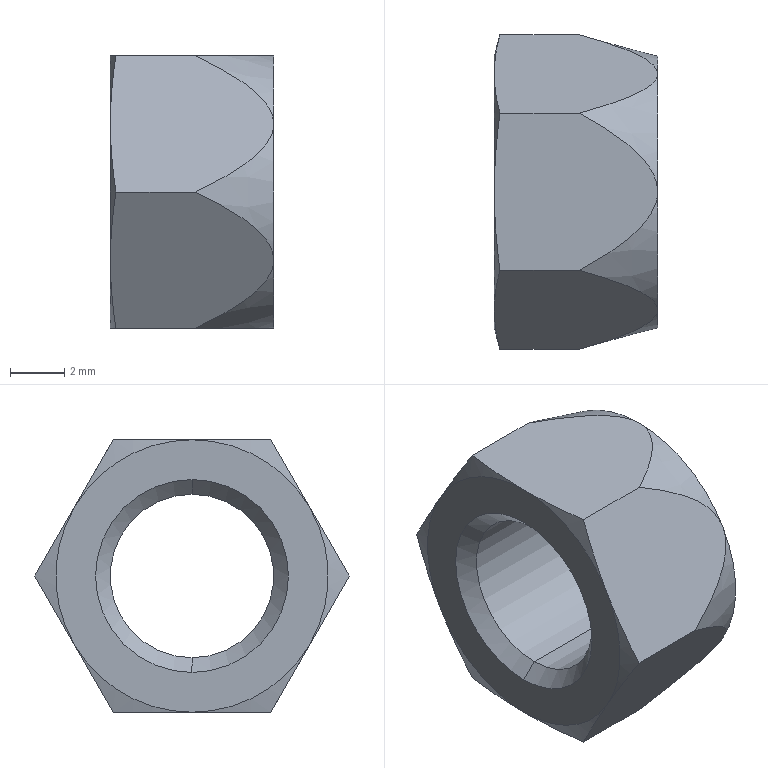Part | STEP file | Microwave Drying Flat Conveyor-nut_gb_t_6185_1_m6 | 1 solid | 26 faces | box 6 x 11.547 x 10 mm | volume 336.581 mm3 | cone 16 | plane 8 | cylinder 2 | commonest cylinder face diameters 6 x2
STEP:
#1=CARTESIAN_POINT('',(0.5413,0.,-3.));
#2=VERTEX_POINT('',#1);
#3=CARTESIAN_POINT('',(0.5413,0.,3.));
#4=VERTEX_POINT('',#3);
#5=CARTESIAN_POINT('',(0.5413,0.,0.));
#6=DIRECTION('',(-1.,0.,0.));
#7=DIRECTION('',(0.,0.,1.));
#8=AXIS2_PLACEMENT_3D('',#5,#6,#7);
#9=CIRCLE('',#8,3.);
#10=EDGE_CURVE('',#2,#4,#9,.T.);
#11=ORIENTED_EDGE('',*,*,#10,.F.);
#12=CARTESIAN_POINT('',(0.,0.,-3.541));
#13=VERTEX_POINT('',#12);
#14=CARTESIAN_POINT('',(0.,0.,-3.541));
#15=DIRECTION('',(-0.7071,0.,-0.7071));
#16=VECTOR('',#15,1000.);
#17=LINE('',#14,#16);
#18=EDGE_CURVE('',#2,#13,#17,.T.);
#19=ORIENTED_EDGE('',*,*,#18,.T.);
#20=CARTESIAN_POINT('',(0.,0.,3.541));
#21=VERTEX_POINT('',#20);
#22=CARTESIAN_POINT('',(0.,0.,0.));
#23=DIRECTION('',(-1.,0.,0.));
#24=DIRECTION('',(0.,0.,1.));
#25=AXIS2_PLACEMENT_3D('',#22,#23,#24);
#26=CIRCLE('',#25,3.541);
#27=EDGE_CURVE('',#13,#21,#26,.T.);
#28=ORIENTED_EDGE('',*,*,#27,.T.);
#29=CARTESIAN_POINT('',(0.,0.,3.541));
#30=DIRECTION('',(-0.7071,0.,0.7071));
#31=VECTOR('',#30,1000.);
#32=LINE('',#29,#31);
#33=EDGE_CURVE('',#4,#21,#32,.T.);
#34=ORIENTED_EDGE('',*,*,#33,.F.);
#35=EDGE_LOOP('',(#11,#19,#28,#34));
#36=FACE_OUTER_BOUND('',#35,.T.);
#37=CARTESIAN_POINT('',(0.,0.,0.));
#38=DIRECTION('',(-1.,0.,0.));
#39=DIRECTION('',(0.,0.,1.));
#40=AXIS2_PLACEMENT_3D('',#37,#38,#39);
#41=CONICAL_SURFACE('',#40,3.541,0.7854);
#42=ADVANCED_FACE('',(#36),#41,.F.);
#43=CARTESIAN_POINT('',(5.459,0.,-3.));
#44=VERTEX_POINT('',#43);
#45=CARTESIAN_POINT('',(5.459,0.,3.));
#46=VERTEX_POINT('',#45);
#47=CARTESIAN_POINT('',(5.459,0.,0.));
#48=DIRECTION('',(-1.,0.,0.));
#49=DIRECTION('',(0.,0.,1.));
#50=AXIS2_PLACEMENT_3D('',#47,#48,#49);
#51=CIRCLE('',#50,3.);
#52=EDGE_CURVE('',#44,#46,#51,.T.);
#53=ORIENTED_EDGE('',*,*,#52,.F.);
#54=CARTESIAN_POINT('',(0.,0.,-3.));
#55=DIRECTION('',(-1.,0.,0.));
#56=VECTOR('',#55,1000.);
#57=LINE('',#54,#56);
#58=EDGE_CURVE('',#44,#2,#57,.T.);
#59=ORIENTED_EDGE('',*,*,#58,.T.);
#60=ORIENTED_EDGE('',*,*,#10,.T.);
#61=CARTESIAN_POINT('',(0.,0.,3.));
#62=DIRECTION('',(-1.,0.,0.));
#63=VECTOR('',#62,1000.);
#64=LINE('',#61,#63);
#65=EDGE_CURVE('',#46,#4,#64,.T.);
#66=ORIENTED_EDGE('',*,*,#65,.F.);
#67=EDGE_LOOP('',(#53,#59,#60,#66));
#68=FACE_OUTER_BOUND('',#67,.T.);
#69=CARTESIAN_POINT('',(0.,0.,0.));
#70=DIRECTION('',(-1.,0.,0.));
#71=DIRECTION('',(0.,0.,1.));
#72=AXIS2_PLACEMENT_3D('',#69,#70,#71);
#73=CYLINDRICAL_SURFACE('',#72,3.);
#74=ADVANCED_FACE('',(#68),#73,.F.);
#75=ORIENTED_EDGE('',*,*,#52,.T.);
#76=CARTESIAN_POINT('',(6.,0.,3.541));
#77=VERTEX_POINT('',#76);
#78=CARTESIAN_POINT('',(5.459,0.,3.));
#79=DIRECTION('',(0.7071,0.,0.7071));
#80=VECTOR('',#79,1000.);
#81=LINE('',#78,#80);
#82=EDGE_CURVE('',#46,#77,#81,.T.);
#83=ORIENTED_EDGE('',*,*,#82,.T.);
#84=CARTESIAN_POINT('',(6.,0.,-3.541));
#85=VERTEX_POINT('',#84);
#86=CARTESIAN_POINT('',(6.,0.,0.));
#87=DIRECTION('',(-1.,0.,0.));
#88=DIRECTION('',(0.,0.,1.));
#89=AXIS2_PLACEMENT_3D('',#86,#87,#88);
#90=CIRCLE('',#89,3.541);
#91=EDGE_CURVE('',#85,#77,#90,.T.);
#92=ORIENTED_EDGE('',*,*,#91,.F.);
#93=CARTESIAN_POINT('',(5.459,0.,-3.));
#94=DIRECTION('',(0.7071,0.,-0.7071));
#95=VECTOR('',#94,1000.);
#96=LINE('',#93,#95);
#97=EDGE_CURVE('',#44,#85,#96,.T.);
#98=ORIENTED_EDGE('',*,*,#97,.F.);
#99=EDGE_LOOP('',(#75,#83,#92,#98));
#100=FACE_OUTER_BOUND('',#99,.T.);
#101=CARTESIAN_POINT('',(5.459,0.,0.));
#102=DIRECTION('',(1.,0.,0.));
#103=DIRECTION('',(0.,0.,-1.));
#104=AXIS2_PLACEMENT_3D('',#101,#102,#103);
#105=CONICAL_SURFACE('',#104,3.,0.7854);
#106=ADVANCED_FACE('',(#100),#105,.F.);
#107=CARTESIAN_POINT('',(3.113,2.887,-5.));
#108=VERTEX_POINT('',#107);
#109=CARTESIAN_POINT('',(6.,0.,-5.));
#110=VERTEX_POINT('',#109);
#111=CARTESIAN_POINT('',(3.113,2.887,-5.));
#112=CARTESIAN_POINT('',(3.423,2.721,-5.));
#113=CARTESIAN_POINT('',(3.729,2.547,-5.));
#114=CARTESIAN_POINT('',(4.326,2.172,-5.));
#115=CARTESIAN_POINT('',(4.619,1.97,-5.));
#116=CARTESIAN_POINT('',(5.033,1.634,-5.));
#117=CARTESIAN_POINT('',(5.165,1.517,-5.));
#118=CARTESIAN_POINT('',(5.416,1.267,-5.));
#119=CARTESIAN_POINT('',(5.534,1.133,-5.));
#120=CARTESIAN_POINT('',(5.744,0.8433,-5.));
#121=CARTESIAN_POINT('',(5.833,0.69,-5.));
#122=CARTESIAN_POINT('',(5.963,0.3563,-5.));
#123=CARTESIAN_POINT('',(6.,0.1802,-5.));
#124=CARTESIAN_POINT('',(6.,0.,-5.));
#125=B_SPLINE_CURVE_WITH_KNOTS('',3,(#111,#112,#113,#114,#115,#116,#117,#118,#119,#120,#121,#122,#123,#124),.UNSPECIFIED.,.F.,.F.,(4,2,2,2,2,2,4),(0.002995,0.004049,0.005104,0.005631,0.006158,0.006685,0.007212),.UNSPECIFIED.);
#126=EDGE_CURVE('',#108,#110,#125,.T.);
#127=ORIENTED_EDGE('',*,*,#126,.F.);
#128=CARTESIAN_POINT('',(6.,4.33,-2.5));
#129=VERTEX_POINT('',#128);
#130=CARTESIAN_POINT('',(6.,4.33,-2.5));
#131=CARTESIAN_POINT('',(6.,4.241,-2.654));
#132=CARTESIAN_POINT('',(5.963,4.152,-2.808));
#133=CARTESIAN_POINT('',(5.835,3.987,-3.095));
#134=CARTESIAN_POINT('',(5.745,3.909,-3.229));
#135=CARTESIAN_POINT('',(5.432,3.693,-3.604));
#136=CARTESIAN_POINT('',(5.174,3.571,-3.816));
#137=CARTESIAN_POINT('',(4.623,3.346,-4.204));
#138=CARTESIAN_POINT('',(4.331,3.246,-4.378));
#139=CARTESIAN_POINT('',(3.733,3.058,-4.703));
#140=CARTESIAN_POINT('',(3.426,2.97,-4.855));
#141=CARTESIAN_POINT('',(3.113,2.887,-5.));
#142=B_SPLINE_CURVE_WITH_KNOTS('',3,(#130,#131,#132,#133,#134,#135,#136,#137,#138,#139,#140,#141),.UNSPECIFIED.,.F.,.F.,(4,2,2,2,2,4),(0.004244,0.004777,0.005309,0.006373,0.007438,0.008503),.UNSPECIFIED.);
#143=EDGE_CURVE('',#129,#108,#142,.T.);
#144=ORIENTED_EDGE('',*,*,#143,.F.);
#145=CARTESIAN_POINT('',(6.,0.,0.));
#146=DIRECTION('',(-1.,0.,0.));
#147=DIRECTION('',(0.,0.,1.));
#148=AXIS2_PLACEMENT_3D('',#145,#146,#147);
#149=CIRCLE('',#148,5.);
#150=EDGE_CURVE('',#129,#110,#149,.T.);
#151=ORIENTED_EDGE('',*,*,#150,.T.);
#152=EDGE_LOOP('',(#127,#144,#151));
#153=FACE_OUTER_BOUND('',#152,.T.);
#154=CARTESIAN_POINT('',(6.,0.,0.));
#155=DIRECTION('',(-1.,0.,0.));
#156=DIRECTION('',(0.,0.,1.));
#157=AXIS2_PLACEMENT_3D('',#154,#155,#156);
#158=CONICAL_SURFACE('',#157,5.,0.2618);
#159=ADVANCED_FACE('',(#153),#158,.T.);
#160=CARTESIAN_POINT('',(3.113,-2.887,-5.));
#161=VERTEX_POINT('',#160);
#162=CARTESIAN_POINT('',(6.,0.,-5.));
#163=CARTESIAN_POINT('',(6.,-0.1814,-5.));
#164=CARTESIAN_POINT('',(5.962,-0.3586,-5.));
#165=CARTESIAN_POINT('',(5.831,-0.6949,-5.));
#166=CARTESIAN_POINT('',(5.74,-0.8495,-5.));
#167=CARTESIAN_POINT('',(5.527,-1.142,-5.));
#168=CARTESIAN_POINT('',(5.409,-1.274,-5.));
#169=CARTESIAN_POINT('',(5.16,-1.522,-5.));
#170=CARTESIAN_POINT('',(5.028,-1.638,-5.));
#171=CARTESIAN_POINT('',(4.62,-1.969,-5.));
#172=CARTESIAN_POINT('',(4.33,-2.169,-5.));
#173=CARTESIAN_POINT('',(3.731,-2.545,-5.));
#174=CARTESIAN_POINT('',(3.423,-2.721,-5.));
#175=CARTESIAN_POINT('',(3.113,-2.887,-5.));
#176=B_SPLINE_CURVE_WITH_KNOTS('',3,(#162,#163,#164,#165,#166,#167,#168,#169,#170,#171,#172,#173,#174,#175),.UNSPECIFIED.,.F.,.F.,(4,2,2,2,2,2,4),(0.007212,0.007743,0.008274,0.008805,0.009335,0.0104,0.01146),.UNSPECIFIED.);
#177=EDGE_CURVE('',#110,#161,#176,.T.);
#178=ORIENTED_EDGE('',*,*,#177,.F.);
#179=CARTESIAN_POINT('',(6.,-4.33,-2.5));
#180=VERTEX_POINT('',#179);
#181=CARTESIAN_POINT('',(6.,0.,0.));
#182=DIRECTION('',(-1.,0.,0.));
#183=DIRECTION('',(0.,0.,1.));
#184=AXIS2_PLACEMENT_3D('',#181,#182,#183);
#185=CIRCLE('',#184,5.);
#186=EDGE_CURVE('',#110,#180,#185,.T.);
#187=ORIENTED_EDGE('',*,*,#186,.T.);
#188=CARTESIAN_POINT('',(3.113,-2.887,-5.));
#189=CARTESIAN_POINT('',(3.426,-2.97,-4.855));
#190=CARTESIAN_POINT('',(3.733,-3.058,-4.703));
#191=CARTESIAN_POINT('',(4.332,-3.246,-4.377));
#192=CARTESIAN_POINT('',(4.625,-3.347,-4.203));
#193=CARTESIAN_POINT('',(5.037,-3.515,-3.912));
#194=CARTESIAN_POINT('',(5.17,-3.574,-3.81));
#195=CARTESIAN_POINT('',(5.42,-3.699,-3.593));
#196=CARTESIAN_POINT('',(5.539,-3.766,-3.476));
#197=CARTESIAN_POINT('',(5.745,-3.91,-3.228));
#198=CARTESIAN_POINT('',(5.835,-3.987,-3.094));
#199=CARTESIAN_POINT('',(5.931,-4.111,-2.879));
#200=CARTESIAN_POINT('',(5.956,-4.154,-2.805));
#201=CARTESIAN_POINT('',(5.991,-4.241,-2.655));
#202=CARTESIAN_POINT('',(6.,-4.286,-2.577));
#203=CARTESIAN_POINT('',(6.,-4.33,-2.5));
#204=B_SPLINE_CURVE_WITH_KNOTS('',3,(#188,#189,#190,#191,#192,#193,#194,#195,#196,#197,#198,#199,#200,#201,#202,#203),.UNSPECIFIED.,.F.,.F.,(4,2,2,2,2,2,2,4),(0.000000005,0.001061,0.002122,0.002653,0.003183,0.003714,0.003979,0.004244),.UNSPECIFIED.);
#205=EDGE_CURVE('',#161,#180,#204,.T.);
#206=ORIENTED_EDGE('',*,*,#205,.F.);
#207=EDGE_LOOP('',(#178,#187,#206));
#208=FACE_OUTER_BOUND('',#207,.T.);
#209=CARTESIAN_POINT('',(6.,0.,0.));
#210=DIRECTION('',(-1.,0.,0.));
#211=DIRECTION('',(0.,0.,1.));
#212=AXIS2_PLACEMENT_3D('',#209,#210,#211);
#213=CONICAL_SURFACE('',#212,5.,0.2618);
#214=ADVANCED_FACE('',(#208),#213,.T.);
#215=CARTESIAN_POINT('',(3.113,-5.774,0.));
#216=VERTEX_POINT('',#215);
#217=CARTESIAN_POINT('',(6.,-4.33,-2.5));
#218=CARTESIAN_POINT('',(6.,-4.419,-2.346));
#219=CARTESIAN_POINT('',(5.963,-4.508,-2.192));
#220=CARTESIAN_POINT('',(5.835,-4.674,-1.905));
#221=CARTESIAN_POINT('',(5.745,-4.751,-1.771));
#222=CARTESIAN_POINT('',(5.432,-4.968,-1.396));
#223=CARTESIAN_POINT('',(5.174,-5.09,-1.184));
#224=CARTESIAN_POINT('',(4.623,-5.314,-0.7959));
#225=CARTESIAN_POINT('',(4.331,-5.414,-0.6225));
#226=CARTESIAN_POINT('',(3.733,-5.602,-0.2968));
#227=CARTESIAN_POINT('',(3.426,-5.69,-0.145));
#228=CARTESIAN_POINT('',(3.113,-5.774,0.));
#229=B_SPLINE_CURVE_WITH_KNOTS('',3,(#217,#218,#219,#220,#221,#222,#223,#224,#225,#226,#227,#228),.UNSPECIFIED.,.F.,.F.,(4,2,2,2,2,4),(0.004244,0.004777,0.005309,0.006373,0.007438,0.008503),.UNSPECIFIED.);
#230=EDGE_CURVE('',#180,#216,#229,.T.);
#231=ORIENTED_EDGE('',*,*,#230,.F.);
#232=CARTESIAN_POINT('',(6.,-4.33,2.5));
#233=VERTEX_POINT('',#232);
#234=CARTESIAN_POINT('',(6.,0.,0.));
#235=DIRECTION('',(-1.,0.,0.));
#236=DIRECTION('',(0.,0.,1.));
#237=AXIS2_PLACEMENT_3D('',#234,#235,#236);
#238=CIRCLE('',#237,5.);
#239=EDGE_CURVE('',#180,#233,#238,.T.);
#240=ORIENTED_EDGE('',*,*,#239,.T.);
#241=CARTESIAN_POINT('',(3.113,-5.774,0.));
#242=CARTESIAN_POINT('',(3.426,-5.69,0.145));
#243=CARTESIAN_POINT('',(3.733,-5.602,0.2969));
#244=CARTESIAN_POINT('',(4.332,-5.414,0.623));
#245=CARTESIAN_POINT('',(4.625,-5.313,0.7973));
#246=CARTESIAN_POINT('',(5.037,-5.145,1.088));
#247=CARTESIAN_POINT('',(5.17,-5.086,1.19));
#248=CARTESIAN_POINT('',(5.42,-4.961,1.407));
#249=CARTESIAN_POINT('',(5.539,-4.894,1.524));
#250=CARTESIAN_POINT('',(5.745,-4.751,1.772));
#251=CARTESIAN_POINT('',(5.835,-4.673,1.906));
#252=CARTESIAN_POINT('',(5.931,-4.549,2.121));
#253=CARTESIAN_POINT('',(5.956,-4.506,2.195));
#254=CARTESIAN_POINT('',(5.991,-4.419,2.345));
#255=CARTESIAN_POINT('',(6.,-4.374,2.423));
#256=CARTESIAN_POINT('',(6.,-4.33,2.5));
#257=B_SPLINE_CURVE_WITH_KNOTS('',3,(#241,#242,#243,#244,#245,#246,#247,#248,#249,#250,#251,#252,#253,#254,#255,#256),.UNSPECIFIED.,.F.,.F.,(4,2,2,2,2,2,2,4),(0.000000005,0.001061,0.002122,0.002653,0.003183,0.003714,0.003979,0.004244),.UNSPECIFIED.);
#258=EDGE_CURVE('',#216,#233,#257,.T.);
#259=ORIENTED_EDGE('',*,*,#258,.F.);
#260=EDGE_LOOP('',(#231,#240,#259));
#261=FACE_OUTER_BOUND('',#260,.T.);
#262=CARTESIAN_POINT('',(6.,0.,0.));
#263=DIRECTION('',(-1.,0.,0.));
#264=DIRECTION('',(0.,0.,1.));
#265=AXIS2_PLACEMENT_3D('',#262,#263,#264);
#266=CONICAL_SURFACE('',#265,5.,0.2618);
#267=ADVANCED_FACE('',(#261),#266,.T.);
#268=CARTESIAN_POINT('',(3.113,5.774,0.));
#269=VERTEX_POINT('',#268);
#270=CARTESIAN_POINT('',(3.113,5.774,0.));
#271=CARTESIAN_POINT('',(3.426,5.69,-0.145));
#272=CARTESIAN_POINT('',(3.733,5.602,-0.2969));
#273=CARTESIAN_POINT('',(4.332,5.414,-0.623));
#274=CARTESIAN_POINT('',(4.625,5.313,-0.7973));
#275=CARTESIAN_POINT('',(5.037,5.145,-1.088));
#276=CARTESIAN_POINT('',(5.17,5.086,-1.19));
#277=CARTESIAN_POINT('',(5.42,4.961,-1.407));
#278=CARTESIAN_POINT('',(5.539,4.894,-1.524));
#279=CARTESIAN_POINT('',(5.745,4.751,-1.772));
#280=CARTESIAN_POINT('',(5.835,4.673,-1.906));
#281=CARTESIAN_POINT('',(5.931,4.549,-2.121));
#282=CARTESIAN_POINT('',(5.956,4.506,-2.195));
#283=CARTESIAN_POINT('',(5.991,4.419,-2.345));
#284=CARTESIAN_POINT('',(6.,4.374,-2.423));
#285=CARTESIAN_POINT('',(6.,4.33,-2.5));
#286=B_SPLINE_CURVE_WITH_KNOTS('',3,(#270,#271,#272,#273,#274,#275,#276,#277,#278,#279,#280,#281,#282,#283,#284,#285),.UNSPECIFIED.,.F.,.F.,(4,2,2,2,2,2,2,4),(0.000000005,0.001061,0.002122,0.002653,0.003183,0.003714,0.003979,0.004244),.UNSPECIFIED.);
#287=EDGE_CURVE('',#269,#129,#286,.T.);
#288=ORIENTED_EDGE('',*,*,#287,.F.);
#289=CARTESIAN_POINT('',(6.,4.33,2.5));
#290=VERTEX_POINT('',#289);
#291=CARTESIAN_POINT('',(6.,4.33,2.5));
#292=CARTESIAN_POINT('',(6.,4.419,2.346));
#293=CARTESIAN_POINT('',(5.963,4.508,2.192));
#294=CARTESIAN_POINT('',(5.835,4.674,1.905));
#295=CARTESIAN_POINT('',(5.745,4.751,1.771));
#296=CARTESIAN_POINT('',(5.432,4.968,1.396));
#297=CARTESIAN_POINT('',(5.174,5.09,1.184));
#298=CARTESIAN_POINT('',(4.623,5.314,0.7959));
#299=CARTESIAN_POINT('',(4.331,5.414,0.6225));
#300=CARTESIAN_POINT('',(3.733,5.602,0.2968));
#301=CARTESIAN_POINT('',(3.426,5.69,0.145));
#302=CARTESIAN_POINT('',(3.113,5.774,0.));
#303=B_SPLINE_CURVE_WITH_KNOTS('',3,(#291,#292,#293,#294,#295,#296,#297,#298,#299,#300,#301,#302),.UNSPECIFIED.,.F.,.F.,(4,2,2,2,2,4),(0.004244,0.004777,0.005309,0.006373,0.007438,0.008503),.UNSPECIFIED.);
#304=EDGE_CURVE('',#290,#269,#303,.T.);
#305=ORIENTED_EDGE('',*,*,#304,.F.);
#306=CARTESIAN_POINT('',(6.,0.,0.));
#307=DIRECTION('',(-1.,0.,0.));
#308=DIRECTION('',(0.,0.,1.));
#309=AXIS2_PLACEMENT_3D('',#306,#307,#308);
#310=CIRCLE('',#309,5.);
#311=EDGE_CURVE('',#290,#129,#310,.T.);
#312=ORIENTED_EDGE('',*,*,#311,.T.);
#313=EDGE_LOOP('',(#288,#305,#312));
#314=FACE_OUTER_BOUND('',#313,.T.);
#315=CARTESIAN_POINT('',(6.,0.,0.));
#316=DIRECTION('',(-1.,0.,0.));
#317=DIRECTION('',(0.,0.,1.));
#318=AXIS2_PLACEMENT_3D('',#315,#316,#317);
#319=CONICAL_SURFACE('',#318,5.,0.2618);
#320=ADVANCED_FACE('',(#314),#319,.T.);
#321=CARTESIAN_POINT('',(3.113,-2.887,5.));
#322=VERTEX_POINT('',#321);
#323=CARTESIAN_POINT('',(6.,-4.33,2.5));
#324=CARTESIAN_POINT('',(6.,-4.241,2.654));
#325=CARTESIAN_POINT('',(5.963,-4.152,2.808));
#326=CARTESIAN_POINT('',(5.835,-3.987,3.095));
#327=CARTESIAN_POINT('',(5.745,-3.909,3.229));
#328=CARTESIAN_POINT('',(5.432,-3.693,3.604));
#329=CARTESIAN_POINT('',(5.174,-3.571,3.816));
#330=CARTESIAN_POINT('',(4.623,-3.346,4.204));
#331=CARTESIAN_POINT('',(4.331,-3.246,4.378));
#332=CARTESIAN_POINT('',(3.733,-3.058,4.703));
#333=CARTESIAN_POINT('',(3.426,-2.97,4.855));
#334=CARTESIAN_POINT('',(3.113,-2.887,5.));
#335=B_SPLINE_CURVE_WITH_KNOTS('',3,(#323,#324,#325,#326,#327,#328,#329,#330,#331,#332,#333,#334),.UNSPECIFIED.,.F.,.F.,(4,2,2,2,2,4),(0.004244,0.004777,0.005309,0.006373,0.007438,0.008503),.UNSPECIFIED.);
#336=EDGE_CURVE('',#233,#322,#335,.T.);
#337=ORIENTED_EDGE('',*,*,#336,.F.);
#338=CARTESIAN_POINT('',(6.,0.,5.));
#339=VERTEX_POINT('',#338);
#340=CARTESIAN_POINT('',(6.,0.,0.));
#341=DIRECTION('',(-1.,0.,0.));
#342=DIRECTION('',(0.,0.,1.));
#343=AXIS2_PLACEMENT_3D('',#340,#341,#342);
#344=CIRCLE('',#343,5.);
#345=EDGE_CURVE('',#233,#339,#344,.T.);
#346=ORIENTED_EDGE('',*,*,#345,.T.);
#347=CARTESIAN_POINT('',(3.113,-2.887,5.));
#348=CARTESIAN_POINT('',(3.423,-2.721,5.));
#349=CARTESIAN_POINT('',(3.731,-2.545,5.));
#350=CARTESIAN_POINT('',(4.33,-2.169,5.));
#351=CARTESIAN_POINT('',(4.62,-1.969,5.));
#352=CARTESIAN_POINT('',(5.028,-1.638,5.));
#353=CARTESIAN_POINT('',(5.16,-1.522,5.));
#354=CARTESIAN_POINT('',(5.409,-1.274,5.));
#355=CARTESIAN_POINT('',(5.527,-1.142,5.));
#356=CARTESIAN_POINT('',(5.74,-0.8495,5.));
#357=CARTESIAN_POINT('',(5.831,-0.6949,5.));
#358=CARTESIAN_POINT('',(5.962,-0.3586,5.));
#359=CARTESIAN_POINT('',(6.,-0.1814,5.));
#360=CARTESIAN_POINT('',(6.,0.,5.));
#361=B_SPLINE_CURVE_WITH_KNOTS('',3,(#347,#348,#349,#350,#351,#352,#353,#354,#355,#356,#357,#358,#359,#360),.UNSPECIFIED.,.F.,.F.,(4,2,2,2,2,2,4),(0.008,0.009052,0.0101,0.01063,0.01115,0.01168,0.01221),.UNSPECIFIED.);
#362=EDGE_CURVE('',#322,#339,#361,.T.);
#363=ORIENTED_EDGE('',*,*,#362,.F.);
#364=EDGE_LOOP('',(#337,#346,#363));
#365=FACE_OUTER_BOUND('',#364,.T.);
#366=CARTESIAN_POINT('',(6.,0.,0.));
#367=DIRECTION('',(-1.,0.,0.));
#368=DIRECTION('',(0.,0.,1.));
#369=AXIS2_PLACEMENT_3D('',#366,#367,#368);
#370=CONICAL_SURFACE('',#369,5.,0.2618);
#371=ADVANCED_FACE('',(#365),#370,.T.);
#372=CARTESIAN_POINT('',(3.113,2.887,5.));
#373=VERTEX_POINT('',#372);
#374=CARTESIAN_POINT('',(3.113,2.887,5.));
#375=CARTESIAN_POINT('',(3.426,2.97,4.855));
#376=CARTESIAN_POINT('',(3.733,3.058,4.703));
#377=CARTESIAN_POINT('',(4.332,3.246,4.377));
#378=CARTESIAN_POINT('',(4.625,3.347,4.203));
#379=CARTESIAN_POINT('',(5.037,3.515,3.912));
#380=CARTESIAN_POINT('',(5.17,3.574,3.81));
#381=CARTESIAN_POINT('',(5.42,3.699,3.593));
#382=CARTESIAN_POINT('',(5.539,3.766,3.476));
#383=CARTESIAN_POINT('',(5.745,3.91,3.228));
#384=CARTESIAN_POINT('',(5.835,3.987,3.094));
#385=CARTESIAN_POINT('',(5.931,4.111,2.879));
#386=CARTESIAN_POINT('',(5.956,4.154,2.805));
#387=CARTESIAN_POINT('',(5.991,4.241,2.655));
#388=CARTESIAN_POINT('',(6.,4.286,2.577));
#389=CARTESIAN_POINT('',(6.,4.33,2.5));
#390=B_SPLINE_CURVE_WITH_KNOTS('',3,(#374,#375,#376,#377,#378,#379,#380,#381,#382,#383,#384,#385,#386,#387,#388,#389),.UNSPECIFIED.,.F.,.F.,(4,2,2,2,2,2,2,4),(0.000000005,0.001061,0.002122,0.002653,0.003183,0.003714,0.003979,0.004244),.UNSPECIFIED.);
#391=EDGE_CURVE('',#373,#290,#390,.T.);
#392=ORIENTED_EDGE('',*,*,#391,.F.);
#393=CARTESIAN_POINT('',(6.,0.,5.));
#394=CARTESIAN_POINT('',(6.,0.1802,5.));
#395=CARTESIAN_POINT('',(5.963,0.3563,5.));
#396=CARTESIAN_POINT('',(5.833,0.69,5.));
#397=CARTESIAN_POINT('',(5.744,0.8433,5.));
#398=CARTESIAN_POINT('',(5.534,1.133,5.));
#399=CARTESIAN_POINT('',(5.416,1.267,5.));
#400=CARTESIAN_POINT('',(5.165,1.517,5.));
#401=CARTESIAN_POINT('',(5.033,1.634,5.));
#402=CARTESIAN_POINT('',(4.619,1.97,5.));
#403=CARTESIAN_POINT('',(4.326,2.172,5.));
#404=CARTESIAN_POINT('',(3.729,2.547,5.));
#405=CARTESIAN_POINT('',(3.423,2.721,5.));
#406=CARTESIAN_POINT('',(3.113,2.887,5.));
#407=B_SPLINE_CURVE_WITH_KNOTS('',3,(#393,#394,#395,#396,#397,#398,#399,#400,#401,#402,#403,#404,#405,#406),.UNSPECIFIED.,.F.,.F.,(4,2,2,2,2,2,4),(0.01221,0.01273,0.01325,0.01377,0.01429,0.01534,0.01638),.UNSPECIFIED.);
#408=EDGE_CURVE('',#339,#373,#407,.T.);
#409=ORIENTED_EDGE('',*,*,#408,.F.);
#410=CARTESIAN_POINT('',(6.,0.,0.));
#411=DIRECTION('',(-1.,0.,0.));
#412=DIRECTION('',(0.,0.,1.));
#413=AXIS2_PLACEMENT_3D('',#410,#411,#412);
#414=CIRCLE('',#413,5.);
#415=EDGE_CURVE('',#339,#290,#414,.T.);
#416=ORIENTED_EDGE('',*,*,#415,.T.);
#417=EDGE_LOOP('',(#392,#409,#416));
#418=FACE_OUTER_BOUND('',#417,.T.);
#419=CARTESIAN_POINT('',(6.,0.,0.));
#420=DIRECTION('',(-1.,0.,0.));
#421=DIRECTION('',(0.,0.,1.));
#422=AXIS2_PLACEMENT_3D('',#419,#420,#421);
#423=CONICAL_SURFACE('',#422,5.,0.2618);
#424=ADVANCED_FACE('',(#418),#423,.T.);
#425=ORIENTED_EDGE('',*,*,#91,.T.);
#426=CARTESIAN_POINT('',(6.,0.,0.));
#427=DIRECTION('',(-1.,0.,0.));
#428=DIRECTION('',(0.,0.,1.));
#429=AXIS2_PLACEMENT_3D('',#426,#427,#428);
#430=CIRCLE('',#429,3.541);
#431=EDGE_CURVE('',#77,#85,#430,.T.);
#432=ORIENTED_EDGE('',*,*,#431,.T.);
#433=EDGE_LOOP('',(#425,#432));
#434=FACE_BOUND('',#433,.T.);
#435=ORIENTED_EDGE('',*,*,#415,.F.);
#436=ORIENTED_EDGE('',*,*,#345,.F.);
#437=ORIENTED_EDGE('',*,*,#239,.F.);
#438=ORIENTED_EDGE('',*,*,#186,.F.);
#439=ORIENTED_EDGE('',*,*,#150,.F.);
#440=ORIENTED_EDGE('',*,*,#311,.F.);
#441=EDGE_LOOP('',(#435,#436,#437,#438,#439,#440));
#442=FACE_OUTER_BOUND('',#441,.T.);
#443=CARTESIAN_POINT('',(6.,0.,0.));
#444=DIRECTION('',(-1.,0.,0.));
#445=DIRECTION('',(0.,0.,1.));
#446=AXIS2_PLACEMENT_3D('',#443,#444,#445);
#447=PLANE('',#446);
#448=ADVANCED_FACE('',(#434,#442),#447,.F.);
#449=CARTESIAN_POINT('',(0.2073,-5.774,0.));
#450=VERTEX_POINT('',#449);
#451=CARTESIAN_POINT('',(6.6,-5.774,0.));
#452=DIRECTION('',(-1.,0.,0.));
#453=VECTOR('',#452,1000.);
#454=LINE('',#451,#453);
#455=EDGE_CURVE('',#216,#450,#454,.T.);
#456=ORIENTED_EDGE('',*,*,#455,.F.);
#457=ORIENTED_EDGE('',*,*,#258,.T.);
#458=ORIENTED_EDGE('',*,*,#336,.T.);
#459=CARTESIAN_POINT('',(0.2073,-2.887,5.));
#460=VERTEX_POINT('',#459);
#461=CARTESIAN_POINT('',(6.6,-2.887,5.));
#462=DIRECTION('',(-1.,0.,0.));
#463=VECTOR('',#462,1000.);
#464=LINE('',#461,#463);
#465=EDGE_CURVE('',#322,#460,#464,.T.);
#466=ORIENTED_EDGE('',*,*,#465,.T.);
#467=CARTESIAN_POINT('',(0.,-4.33,2.5));
#468=VERTEX_POINT('',#467);
#469=CARTESIAN_POINT('',(0.,-4.33,2.5));
#470=CARTESIAN_POINT('',(0.,-3.849,3.333));
#471=CARTESIAN_POINT('',(0.07834,-3.368,4.167));
#472=CARTESIAN_POINT('',(0.2073,-2.887,5.));
#473=B_SPLINE_CURVE_WITH_KNOTS('',3,(#469,#470,#471,#472),.UNSPECIFIED.,.F.,.F.,(4,4),(0.002887,0.005774),.UNSPECIFIED.);
#474=EDGE_CURVE('',#468,#460,#473,.T.);
#475=ORIENTED_EDGE('',*,*,#474,.F.);
#476=CARTESIAN_POINT('',(0.2073,-5.774,0.));
#477=CARTESIAN_POINT('',(0.07834,-5.292,0.8333));
#478=CARTESIAN_POINT('',(0.,-4.811,1.667));
#479=CARTESIAN_POINT('',(0.,-4.33,2.5));
#480=B_SPLINE_CURVE_WITH_KNOTS('',3,(#476,#477,#478,#479),.UNSPECIFIED.,.F.,.F.,(4,4),(0.000000002,0.002887),.UNSPECIFIED.);
#481=EDGE_CURVE('',#450,#468,#480,.T.);
#482=ORIENTED_EDGE('',*,*,#481,.F.);
#483=EDGE_LOOP('',(#456,#457,#458,#466,#475,#482));
#484=FACE_OUTER_BOUND('',#483,.T.);
#485=CARTESIAN_POINT('',(6.6,-2.887,5.));
#486=DIRECTION('',(0.,0.866,-0.5));
#487=DIRECTION('',(0.,0.5,0.866));
#488=AXIS2_PLACEMENT_3D('',#485,#486,#487);
#489=PLANE('',#488);
#490=ADVANCED_FACE('',(#484),#489,.F.);
#491=CARTESIAN_POINT('',(0.2073,-2.887,-5.));
#492=VERTEX_POINT('',#491);
#493=CARTESIAN_POINT('',(6.6,-2.887,-5.));
#494=DIRECTION('',(-1.,0.,0.));
#495=VECTOR('',#494,1000.);
#496=LINE('',#493,#495);
#497=EDGE_CURVE('',#161,#492,#496,.T.);
#498=ORIENTED_EDGE('',*,*,#497,.F.);
#499=ORIENTED_EDGE('',*,*,#205,.T.);
#500=ORIENTED_EDGE('',*,*,#230,.T.);
#501=ORIENTED_EDGE('',*,*,#455,.T.);
#502=CARTESIAN_POINT('',(0.,-4.33,-2.5));
#503=VERTEX_POINT('',#502);
#504=CARTESIAN_POINT('',(0.,-4.33,-2.5));
#505=CARTESIAN_POINT('',(0.,-4.811,-1.667));
#506=CARTESIAN_POINT('',(0.07834,-5.292,-0.8333));
#507=CARTESIAN_POINT('',(0.2073,-5.774,0.));
#508=B_SPLINE_CURVE_WITH_KNOTS('',3,(#504,#505,#506,#507),.UNSPECIFIED.,.F.,.F.,(4,4),(0.002887,0.005774),.UNSPECIFIED.);
#509=EDGE_CURVE('',#503,#450,#508,.T.);
#510=ORIENTED_EDGE('',*,*,#509,.F.);
#511=CARTESIAN_POINT('',(0.2073,-2.887,-5.));
#512=CARTESIAN_POINT('',(0.07834,-3.368,-4.167));
#513=CARTESIAN_POINT('',(0.,-3.849,-3.333));
#514=CARTESIAN_POINT('',(0.,-4.33,-2.5));
#515=B_SPLINE_CURVE_WITH_KNOTS('',3,(#511,#512,#513,#514),.UNSPECIFIED.,.F.,.F.,(4,4),(0.000000002,0.002887),.UNSPECIFIED.);
#516=EDGE_CURVE('',#492,#503,#515,.T.);
#517=ORIENTED_EDGE('',*,*,#516,.F.);
#518=EDGE_LOOP('',(#498,#499,#500,#501,#510,#517));
#519=FACE_OUTER_BOUND('',#518,.T.);
#520=CARTESIAN_POINT('',(6.6,-5.774,0.));
#521=DIRECTION('',(0.,0.866,0.5));
#522=DIRECTION('',(0.,-0.5,0.866));
#523=AXIS2_PLACEMENT_3D('',#520,#521,#522);
#524=PLANE('',#523);
#525=ADVANCED_FACE('',(#519),#524,.F.);
#526=CARTESIAN_POINT('',(0.2073,2.887,-5.));
#527=VERTEX_POINT('',#526);
#528=CARTESIAN_POINT('',(6.6,2.887,-5.));
#529=DIRECTION('',(-1.,0.,0.));
#530=VECTOR('',#529,1000.);
#531=LINE('',#528,#530);
#532=EDGE_CURVE('',#108,#527,#531,.T.);
#533=ORIENTED_EDGE('',*,*,#532,.F.);
#534=ORIENTED_EDGE('',*,*,#126,.T.);
#535=ORIENTED_EDGE('',*,*,#177,.T.);
#536=ORIENTED_EDGE('',*,*,#497,.T.);
#537=CARTESIAN_POINT('',(0.,0.,-5.));
#538=VERTEX_POINT('',#537);
#539=CARTESIAN_POINT('',(0.,0.,-5.));
#540=CARTESIAN_POINT('',(0.,-0.4805,-5.));
#541=CARTESIAN_POINT('',(0.0189,-0.9615,-5.));
#542=CARTESIAN_POINT('',(0.09045,-1.925,-5.));
#543=CARTESIAN_POINT('',(0.143,-2.407,-5.));
#544=CARTESIAN_POINT('',(0.2073,-2.887,-5.));
#545=B_SPLINE_CURVE_WITH_KNOTS('',3,(#539,#540,#541,#542,#543,#544),.UNSPECIFIED.,.F.,.F.,(4,2,4),(0.01389,0.01534,0.01678),.UNSPECIFIED.);
#546=EDGE_CURVE('',#538,#492,#545,.T.);
#547=ORIENTED_EDGE('',*,*,#546,.F.);
#548=CARTESIAN_POINT('',(0.2073,2.887,-5.));
#549=CARTESIAN_POINT('',(0.07858,1.926,-5.));
#550=CARTESIAN_POINT('',(0.,0.9643,-5.));
#551=CARTESIAN_POINT('',(0.,0.,-5.));
#552=B_SPLINE_CURVE_WITH_KNOTS('',3,(#548,#549,#550,#551),.UNSPECIFIED.,.F.,.F.,(4,4),(0.01098,0.01389),.UNSPECIFIED.);
#553=EDGE_CURVE('',#527,#538,#552,.T.);
#554=ORIENTED_EDGE('',*,*,#553,.F.);
#555=EDGE_LOOP('',(#533,#534,#535,#536,#547,#554));
#556=FACE_OUTER_BOUND('',#555,.T.);
#557=CARTESIAN_POINT('',(6.6,-2.887,-5.));
#558=DIRECTION('',(0.,0.,1.));
#559=DIRECTION('',(0.,-1.,0.));
#560=AXIS2_PLACEMENT_3D('',#557,#558,#559);
#561=PLANE('',#560);
#562=ADVANCED_FACE('',(#556),#561,.F.);
#563=CARTESIAN_POINT('',(0.2073,5.774,0.));
#564=VERTEX_POINT('',#563);
#565=CARTESIAN_POINT('',(6.6,5.774,0.));
#566=DIRECTION('',(-1.,0.,0.));
#567=VECTOR('',#566,1000.);
#568=LINE('',#565,#567);
#569=EDGE_CURVE('',#269,#564,#568,.T.);
#570=ORIENTED_EDGE('',*,*,#569,.F.);
#571=ORIENTED_EDGE('',*,*,#287,.T.);
#572=ORIENTED_EDGE('',*,*,#143,.T.);
#573=ORIENTED_EDGE('',*,*,#532,.T.);
#574=CARTESIAN_POINT('',(0.,4.33,-2.5));
#575=VERTEX_POINT('',#574);
#576=CARTESIAN_POINT('',(0.,4.33,-2.5));
#577=CARTESIAN_POINT('',(0.,3.849,-3.333));
#578=CARTESIAN_POINT('',(0.07834,3.368,-4.167));
#579=CARTESIAN_POINT('',(0.2073,2.887,-5.));
#580=B_SPLINE_CURVE_WITH_KNOTS('',3,(#576,#577,#578,#579),.UNSPECIFIED.,.F.,.F.,(4,4),(0.002887,0.005774),.UNSPECIFIED.);
#581=EDGE_CURVE('',#575,#527,#580,.T.);
#582=ORIENTED_EDGE('',*,*,#581,.F.);
#583=CARTESIAN_POINT('',(0.2073,5.774,0.));
#584=CARTESIAN_POINT('',(0.07834,5.292,-0.8333));
#585=CARTESIAN_POINT('',(0.,4.811,-1.667));
#586=CARTESIAN_POINT('',(0.,4.33,-2.5));
#587=B_SPLINE_CURVE_WITH_KNOTS('',3,(#583,#584,#585,#586),.UNSPECIFIED.,.F.,.F.,(4,4),(0.000000002,0.002887),.UNSPECIFIED.);
#588=EDGE_CURVE('',#564,#575,#587,.T.);
#589=ORIENTED_EDGE('',*,*,#588,.F.);
#590=EDGE_LOOP('',(#570,#571,#572,#573,#582,#589));
#591=FACE_OUTER_BOUND('',#590,.T.);
#592=CARTESIAN_POINT('',(6.6,2.887,-5.));
#593=DIRECTION('',(0.,-0.866,0.5));
#594=DIRECTION('',(0.,-0.5,-0.866));
#595=AXIS2_PLACEMENT_3D('',#592,#593,#594);
#596=PLANE('',#595);
#597=ADVANCED_FACE('',(#591),#596,.F.);
#598=CARTESIAN_POINT('',(0.2073,2.887,5.));
#599=VERTEX_POINT('',#598);
#600=CARTESIAN_POINT('',(6.6,2.887,5.));
#601=DIRECTION('',(-1.,0.,0.));
#602=VECTOR('',#601,1000.);
#603=LINE('',#600,#602);
#604=EDGE_CURVE('',#373,#599,#603,.T.);
#605=ORIENTED_EDGE('',*,*,#604,.F.);
#606=ORIENTED_EDGE('',*,*,#391,.T.);
#607=ORIENTED_EDGE('',*,*,#304,.T.);
#608=ORIENTED_EDGE('',*,*,#569,.T.);
#609=CARTESIAN_POINT('',(0.,4.33,2.5));
#610=VERTEX_POINT('',#609);
#611=CARTESIAN_POINT('',(0.,4.33,2.5));
#612=CARTESIAN_POINT('',(0.,4.811,1.667));
#613=CARTESIAN_POINT('',(0.07834,5.292,0.8333));
#614=CARTESIAN_POINT('',(0.2073,5.774,0.));
#615=B_SPLINE_CURVE_WITH_KNOTS('',3,(#611,#612,#613,#614),.UNSPECIFIED.,.F.,.F.,(4,4),(0.002887,0.005774),.UNSPECIFIED.);
#616=EDGE_CURVE('',#610,#564,#615,.T.);
#617=ORIENTED_EDGE('',*,*,#616,.F.);
#618=CARTESIAN_POINT('',(0.2073,2.887,5.));
#619=CARTESIAN_POINT('',(0.07834,3.368,4.167));
#620=CARTESIAN_POINT('',(0.,3.849,3.333));
#621=CARTESIAN_POINT('',(0.,4.33,2.5));
#622=B_SPLINE_CURVE_WITH_KNOTS('',3,(#618,#619,#620,#621),.UNSPECIFIED.,.F.,.F.,(4,4),(0.000000002,0.002887),.UNSPECIFIED.);
#623=EDGE_CURVE('',#599,#610,#622,.T.);
#624=ORIENTED_EDGE('',*,*,#623,.F.);
#625=EDGE_LOOP('',(#605,#606,#607,#608,#617,#624));
#626=FACE_OUTER_BOUND('',#625,.T.);
#627=CARTESIAN_POINT('',(6.6,5.774,0.));
#628=DIRECTION('',(0.,-0.866,-0.5));
#629=DIRECTION('',(0.,0.5,-0.866));
#630=AXIS2_PLACEMENT_3D('',#627,#628,#629);
#631=PLANE('',#630);
#632=ADVANCED_FACE('',(#626),#631,.F.);
#633=ORIENTED_EDGE('',*,*,#465,.F.);
#634=ORIENTED_EDGE('',*,*,#362,.T.);
#635=ORIENTED_EDGE('',*,*,#408,.T.);
#636=ORIENTED_EDGE('',*,*,#604,.T.);
#637=CARTESIAN_POINT('',(0.,0.,5.));
#638=VERTEX_POINT('',#637);
#639=CARTESIAN_POINT('',(0.,0.,5.));
#640=CARTESIAN_POINT('',(0.,0.9643,5.));
#641=CARTESIAN_POINT('',(0.07858,1.926,5.));
#642=CARTESIAN_POINT('',(0.2073,2.887,5.));
#643=B_SPLINE_CURVE_WITH_KNOTS('',3,(#639,#640,#641,#642),.UNSPECIFIED.,.F.,.F.,(4,4),(0.007731,0.01064),.UNSPECIFIED.);
#644=EDGE_CURVE('',#638,#599,#643,.T.);
#645=ORIENTED_EDGE('',*,*,#644,.F.);
#646=CARTESIAN_POINT('',(0.2073,-2.887,5.));
#647=CARTESIAN_POINT('',(0.143,-2.407,5.));
#648=CARTESIAN_POINT('',(0.09045,-1.925,5.));
#649=CARTESIAN_POINT('',(0.0189,-0.9615,5.));
#650=CARTESIAN_POINT('',(0.,-0.4805,5.));
#651=CARTESIAN_POINT('',(0.,0.,5.));
#652=B_SPLINE_CURVE_WITH_KNOTS('',3,(#646,#647,#648,#649,#650,#651),.UNSPECIFIED.,.F.,.F.,(4,2,4),(0.00483,0.00628,0.007731),.UNSPECIFIED.);
#653=EDGE_CURVE('',#460,#638,#652,.T.);
#654=ORIENTED_EDGE('',*,*,#653,.F.);
#655=EDGE_LOOP('',(#633,#634,#635,#636,#645,#654));
#656=FACE_OUTER_BOUND('',#655,.T.);
#657=CARTESIAN_POINT('',(6.6,2.887,5.));
#658=DIRECTION('',(0.,0.,-1.));
#659=DIRECTION('',(0.,1.,0.));
#660=AXIS2_PLACEMENT_3D('',#657,#658,#659);
#661=PLANE('',#660);
#662=ADVANCED_FACE('',(#656),#661,.F.);
#663=CARTESIAN_POINT('',(0.,0.,0.));
#664=DIRECTION('',(-1.,0.,0.));
#665=DIRECTION('',(0.,0.,1.));
#666=AXIS2_PLACEMENT_3D('',#663,#664,#665);
#667=CIRCLE('',#666,5.);
#668=EDGE_CURVE('',#468,#638,#667,.T.);
#669=ORIENTED_EDGE('',*,*,#668,.F.);
#670=ORIENTED_EDGE('',*,*,#474,.T.);
#671=ORIENTED_EDGE('',*,*,#653,.T.);
#672=EDGE_LOOP('',(#669,#670,#671));
#673=FACE_OUTER_BOUND('',#672,.T.);
#674=CARTESIAN_POINT('',(0.,0.,0.));
#675=DIRECTION('',(1.,0.,0.));
#676=DIRECTION('',(0.,0.,-1.));
#677=AXIS2_PLACEMENT_3D('',#674,#675,#676);
#678=CONICAL_SURFACE('',#677,5.,1.309);
#679=ADVANCED_FACE('',(#673),#678,.T.);
#680=CARTESIAN_POINT('',(0.,0.,0.));
#681=DIRECTION('',(-1.,0.,0.));
#682=DIRECTION('',(0.,0.,1.));
#683=AXIS2_PLACEMENT_3D('',#680,#681,#682);
#684=CIRCLE('',#683,5.);
#685=EDGE_CURVE('',#503,#468,#684,.T.);
#686=ORIENTED_EDGE('',*,*,#685,.F.);
#687=ORIENTED_EDGE('',*,*,#509,.T.);
#688=ORIENTED_EDGE('',*,*,#481,.T.);
#689=EDGE_LOOP('',(#686,#687,#688));
#690=FACE_OUTER_BOUND('',#689,.T.);
#691=CARTESIAN_POINT('',(0.,0.,0.));
#692=DIRECTION('',(1.,0.,0.));
#693=DIRECTION('',(0.,0.,-1.));
#694=AXIS2_PLACEMENT_3D('',#691,#692,#693);
#695=CONICAL_SURFACE('',#694,5.,1.309);
#696=ADVANCED_FACE('',(#690),#695,.T.);
#697=CARTESIAN_POINT('',(0.,0.,0.));
#698=DIRECTION('',(-1.,0.,0.));
#699=DIRECTION('',(0.,0.,1.));
#700=AXIS2_PLACEMENT_3D('',#697,#698,#699);
#701=CIRCLE('',#700,5.);
#702=EDGE_CURVE('',#538,#503,#701,.T.);
#703=ORIENTED_EDGE('',*,*,#702,.F.);
#704=ORIENTED_EDGE('',*,*,#546,.T.);
#705=ORIENTED_EDGE('',*,*,#516,.T.);
#706=EDGE_LOOP('',(#703,#704,#705));
#707=FACE_OUTER_BOUND('',#706,.T.);
#708=CARTESIAN_POINT('',(0.,0.,0.));
#709=DIRECTION('',(1.,0.,0.));
#710=DIRECTION('',(0.,0.,-1.));
#711=AXIS2_PLACEMENT_3D('',#708,#709,#710);
#712=CONICAL_SURFACE('',#711,5.,1.309);
#713=ADVANCED_FACE('',(#707),#712,.T.);
#714=ORIENTED_EDGE('',*,*,#581,.T.);
#715=ORIENTED_EDGE('',*,*,#553,.T.);
#716=CARTESIAN_POINT('',(0.,0.,0.));
#717=DIRECTION('',(-1.,0.,0.));
#718=DIRECTION('',(0.,0.,1.));
#719=AXIS2_PLACEMENT_3D('',#716,#717,#718);
#720=CIRCLE('',#719,5.);
#721=EDGE_CURVE('',#575,#538,#720,.T.);
#722=ORIENTED_EDGE('',*,*,#721,.F.);
#723=EDGE_LOOP('',(#714,#715,#722));
#724=FACE_OUTER_BOUND('',#723,.T.);
#725=CARTESIAN_POINT('',(0.,0.,0.));
#726=DIRECTION('',(1.,0.,0.));
#727=DIRECTION('',(0.,0.,-1.));
#728=AXIS2_PLACEMENT_3D('',#725,#726,#727);
#729=CONICAL_SURFACE('',#728,5.,1.309);
#730=ADVANCED_FACE('',(#724),#729,.T.);
#731=ORIENTED_EDGE('',*,*,#616,.T.);
#732=ORIENTED_EDGE('',*,*,#588,.T.);
#733=CARTESIAN_POINT('',(0.,0.,0.));
#734=DIRECTION('',(-1.,0.,0.));
#735=DIRECTION('',(0.,0.,1.));
#736=AXIS2_PLACEMENT_3D('',#733,#734,#735);
#737=CIRCLE('',#736,5.);
#738=EDGE_CURVE('',#610,#575,#737,.T.);
#739=ORIENTED_EDGE('',*,*,#738,.F.);
#740=EDGE_LOOP('',(#731,#732,#739));
#741=FACE_OUTER_BOUND('',#740,.T.);
#742=CARTESIAN_POINT('',(0.,0.,0.));
#743=DIRECTION('',(1.,0.,0.));
#744=DIRECTION('',(0.,0.,-1.));
#745=AXIS2_PLACEMENT_3D('',#742,#743,#744);
#746=CONICAL_SURFACE('',#745,5.,1.309);
#747=ADVANCED_FACE('',(#741),#746,.T.);
#748=CARTESIAN_POINT('',(0.,0.,0.));
#749=DIRECTION('',(-1.,0.,0.));
#750=DIRECTION('',(0.,0.,1.));
#751=AXIS2_PLACEMENT_3D('',#748,#749,#750);
#752=CIRCLE('',#751,3.541);
#753=EDGE_CURVE('',#21,#13,#752,.T.);
#754=ORIENTED_EDGE('',*,*,#753,.F.);
#755=ORIENTED_EDGE('',*,*,#27,.F.);
#756=EDGE_LOOP('',(#754,#755));
#757=FACE_BOUND('',#756,.T.);
#758=CARTESIAN_POINT('',(0.,0.,0.));
#759=DIRECTION('',(-1.,0.,0.));
#760=DIRECTION('',(0.,0.,1.));
#761=AXIS2_PLACEMENT_3D('',#758,#759,#760);
#762=CIRCLE('',#761,5.);
#763=EDGE_CURVE('',#638,#610,#762,.T.);
#764=ORIENTED_EDGE('',*,*,#763,.T.);
#765=ORIENTED_EDGE('',*,*,#738,.T.);
#766=ORIENTED_EDGE('',*,*,#721,.T.);
#767=ORIENTED_EDGE('',*,*,#702,.T.);
#768=ORIENTED_EDGE('',*,*,#685,.T.);
#769=ORIENTED_EDGE('',*,*,#668,.T.);
#770=EDGE_LOOP('',(#764,#765,#766,#767,#768,#769));
#771=FACE_OUTER_BOUND('',#770,.T.);
#772=CARTESIAN_POINT('',(0.,0.,0.));
#773=DIRECTION('',(-1.,0.,0.));
#774=DIRECTION('',(0.,0.,1.));
#775=AXIS2_PLACEMENT_3D('',#772,#773,#774);
#776=PLANE('',#775);
#777=ADVANCED_FACE('',(#757,#771),#776,.T.);
#778=ORIENTED_EDGE('',*,*,#644,.T.);
#779=ORIENTED_EDGE('',*,*,#623,.T.);
#780=ORIENTED_EDGE('',*,*,#763,.F.);
#781=EDGE_LOOP('',(#778,#779,#780));
#782=FACE_OUTER_BOUND('',#781,.T.);
#783=CARTESIAN_POINT('',(0.,0.,0.));
#784=DIRECTION('',(1.,0.,0.));
#785=DIRECTION('',(0.,0.,-1.));
#786=AXIS2_PLACEMENT_3D('',#783,#784,#785);
#787=CONICAL_SURFACE('',#786,5.,1.309);
#788=ADVANCED_FACE('',(#782),#787,.T.);
#789=ORIENTED_EDGE('',*,*,#82,.F.);
#790=CARTESIAN_POINT('',(5.459,0.,0.));
#791=DIRECTION('',(-1.,0.,0.));
#792=DIRECTION('',(0.,0.,1.));
#793=AXIS2_PLACEMENT_3D('',#790,#791,#792);
#794=CIRCLE('',#793,3.);
#795=EDGE_CURVE('',#46,#44,#794,.T.);
#796=ORIENTED_EDGE('',*,*,#795,.T.);
#797=ORIENTED_EDGE('',*,*,#97,.T.);
#798=ORIENTED_EDGE('',*,*,#431,.F.);
#799=EDGE_LOOP('',(#789,#796,#797,#798));
#800=FACE_OUTER_BOUND('',#799,.T.);
#801=CARTESIAN_POINT('',(5.459,0.,0.));
#802=DIRECTION('',(1.,0.,0.));
#803=DIRECTION('',(0.,0.,-1.));
#804=AXIS2_PLACEMENT_3D('',#801,#802,#803);
#805=CONICAL_SURFACE('',#804,3.,0.7854);
#806=ADVANCED_FACE('',(#800),#805,.F.);
#807=ORIENTED_EDGE('',*,*,#58,.F.);
#808=ORIENTED_EDGE('',*,*,#795,.F.);
#809=ORIENTED_EDGE('',*,*,#65,.T.);
#810=CARTESIAN_POINT('',(0.5413,0.,0.));
#811=DIRECTION('',(-1.,0.,0.));
#812=DIRECTION('',(0.,0.,1.));
#813=AXIS2_PLACEMENT_3D('',#810,#811,#812);
#814=CIRCLE('',#813,3.);
#815=EDGE_CURVE('',#4,#2,#814,.T.);
#816=ORIENTED_EDGE('',*,*,#815,.T.);
#817=EDGE_LOOP('',(#807,#808,#809,#816));
#818=FACE_OUTER_BOUND('',#817,.T.);
#819=CARTESIAN_POINT('',(0.,0.,0.));
#820=DIRECTION('',(-1.,0.,0.));
#821=DIRECTION('',(0.,0.,1.));
#822=AXIS2_PLACEMENT_3D('',#819,#820,#821);
#823=CYLINDRICAL_SURFACE('',#822,3.);
#824=ADVANCED_FACE('',(#818),#823,.F.);
#825=ORIENTED_EDGE('',*,*,#18,.F.);
#826=ORIENTED_EDGE('',*,*,#815,.F.);
#827=ORIENTED_EDGE('',*,*,#33,.T.);
#828=ORIENTED_EDGE('',*,*,#753,.T.);
#829=EDGE_LOOP('',(#825,#826,#827,#828));
#830=FACE_OUTER_BOUND('',#829,.T.);
#831=CARTESIAN_POINT('',(0.,0.,0.));
#832=DIRECTION('',(-1.,0.,0.));
#833=DIRECTION('',(0.,0.,1.));
#834=AXIS2_PLACEMENT_3D('',#831,#832,#833);
#835=CONICAL_SURFACE('',#834,3.541,0.7854);
#836=ADVANCED_FACE('',(#830),#835,.F.);
#837=CLOSED_SHELL('',(#42,#74,#106,#159,#214,#267,#320,#371,#424,#448,#490,#525,#562,#597,#632,#662,#679,#696,#713,#730,#747,#777,#788,#806,#824,#836));
#838=MANIFOLD_SOLID_BREP('',#837);
#839=CARTESIAN_POINT('',(0.,0.,0.));
#840=DIRECTION('',(0.,0.,1.));
#841=DIRECTION('',(1.,0.,0.));
#842=AXIS2_PLACEMENT_3D('',#839,#840,#841);
#843=(LENGTH_UNIT()NAMED_UNIT(*)SI_UNIT(.MILLI.,.METRE.));
#844=UNCERTAINTY_MEASURE_WITH_UNIT(LENGTH_MEASURE(0.00001),#843,'','');
#845=(NAMED_UNIT(*)PLANE_ANGLE_UNIT()SI_UNIT($,.RADIAN.));
#846=(NAMED_UNIT(*)SI_UNIT($,.STERADIAN.)SOLID_ANGLE_UNIT());
#847=(GEOMETRIC_REPRESENTATION_CONTEXT(3)GLOBAL_UNCERTAINTY_ASSIGNED_CONTEXT((#844))GLOBAL_UNIT_ASSIGNED_CONTEXT((#843,#845,#846))REPRESENTATION_CONTEXT('',''));
#848=ADVANCED_BREP_SHAPE_REPRESENTATION('',(#838,#842),#847);